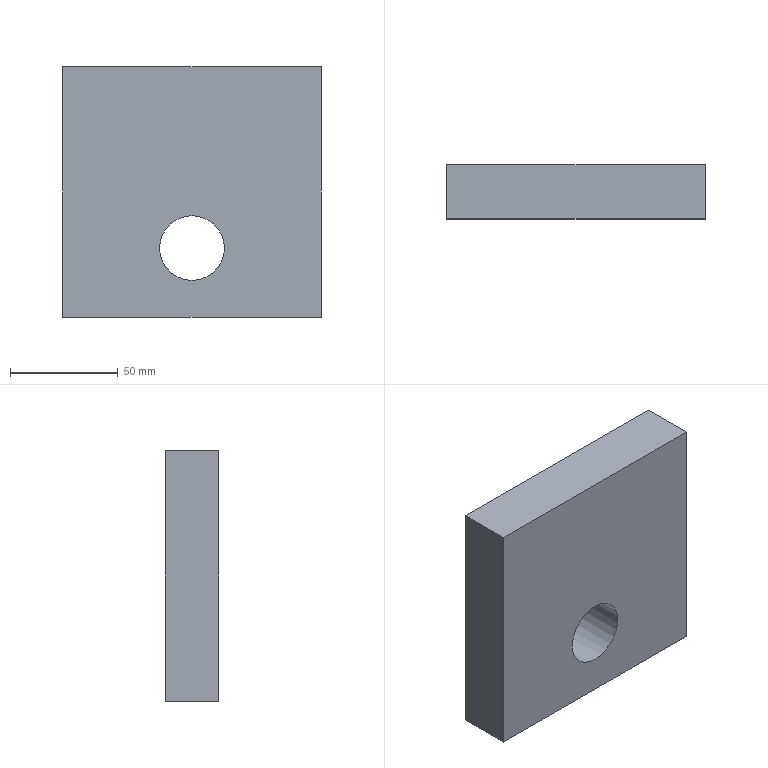Part | NX | features 掩护梁 2 | 1 solid | 7 faces | box 120 x 25 x 116 mm | volume 330329 mm3 | plane 6 | cylinder 1 | commonest cylinder face diameters 30 x1
STEP:
#1=CARTESIAN_POINT('',(-1641.68,3664.947,-172.771));
#2=VERTEX_POINT('',#1);
#3=CARTESIAN_POINT('',(-1641.68,3689.947,-172.771));
#4=VERTEX_POINT('',#3);
#5=CARTESIAN_POINT('',(-1641.68,3689.947,-172.771));
#6=DIRECTION('',(0.,1.,0.));
#7=VECTOR('',#6,1000.);
#8=LINE('',#5,#7);
#9=EDGE_CURVE('',#2,#4,#8,.T.);
#10=ORIENTED_EDGE('',*,*,#9,.F.);
#11=CARTESIAN_POINT('',(-1641.68,3664.947,-288.771));
#12=VERTEX_POINT('',#11);
#13=CARTESIAN_POINT('',(-1641.68,3664.947,-288.771));
#14=DIRECTION('',(0.,0.,1.));
#15=VECTOR('',#14,1000.);
#16=LINE('',#13,#15);
#17=EDGE_CURVE('',#12,#2,#16,.T.);
#18=ORIENTED_EDGE('',*,*,#17,.F.);
#19=CARTESIAN_POINT('',(-1641.68,3689.947,-288.771));
#20=VERTEX_POINT('',#19);
#21=CARTESIAN_POINT('',(-1641.68,3689.947,-288.771));
#22=DIRECTION('',(0.,1.,0.));
#23=VECTOR('',#22,1000.);
#24=LINE('',#21,#23);
#25=EDGE_CURVE('',#12,#20,#24,.T.);
#26=ORIENTED_EDGE('',*,*,#25,.T.);
#27=CARTESIAN_POINT('',(-1641.68,3689.947,-288.771));
#28=DIRECTION('',(0.,0.,1.));
#29=VECTOR('',#28,1000.);
#30=LINE('',#27,#29);
#31=EDGE_CURVE('',#20,#4,#30,.T.);
#32=ORIENTED_EDGE('',*,*,#31,.T.);
#33=EDGE_LOOP('',(#10,#18,#26,#32));
#34=FACE_BOUND('',#33,.T.);
#35=CARTESIAN_POINT('',(-1641.68,3689.947,-288.771));
#36=DIRECTION('',(1.,0.,0.));
#37=DIRECTION('',(0.,0.,-1.));
#38=AXIS2_PLACEMENT_3D('',#35,#36,#37);
#39=PLANE('',#38);
#40=ADVANCED_FACE('',(#34),#39,.T.);
#41=CARTESIAN_POINT('',(-1701.68,3664.947,-271.771));
#42=VERTEX_POINT('',#41);
#43=CARTESIAN_POINT('',(-1701.68,3664.947,-256.771));
#44=DIRECTION('',(0.,-1.,0.));
#45=DIRECTION('',(0.,0.,-1.));
#46=AXIS2_PLACEMENT_3D('',#43,#44,#45);
#47=CIRCLE('',#46,15.);
#48=EDGE_CURVE('',#42,#42,#47,.T.);
#49=ORIENTED_EDGE('',*,*,#48,.F.);
#50=EDGE_LOOP('',(#49));
#51=FACE_BOUND('',#50,.T.);
#52=CARTESIAN_POINT('',(-1761.68,3664.947,-172.771));
#53=VERTEX_POINT('',#52);
#54=CARTESIAN_POINT('',(-1641.68,3664.947,-172.771));
#55=DIRECTION('',(1.,0.,0.));
#56=VECTOR('',#55,1000.);
#57=LINE('',#54,#56);
#58=EDGE_CURVE('',#53,#2,#57,.T.);
#59=ORIENTED_EDGE('',*,*,#58,.F.);
#60=CARTESIAN_POINT('',(-1761.68,3664.947,-288.771));
#61=VERTEX_POINT('',#60);
#62=CARTESIAN_POINT('',(-1761.68,3664.947,-288.771));
#63=DIRECTION('',(0.,0.,1.));
#64=VECTOR('',#63,1000.);
#65=LINE('',#62,#64);
#66=EDGE_CURVE('',#61,#53,#65,.T.);
#67=ORIENTED_EDGE('',*,*,#66,.F.);
#68=CARTESIAN_POINT('',(-1641.68,3664.947,-288.771));
#69=DIRECTION('',(1.,0.,0.));
#70=VECTOR('',#69,1000.);
#71=LINE('',#68,#70);
#72=EDGE_CURVE('',#61,#12,#71,.T.);
#73=ORIENTED_EDGE('',*,*,#72,.T.);
#74=ORIENTED_EDGE('',*,*,#17,.T.);
#75=EDGE_LOOP('',(#59,#67,#73,#74));
#76=FACE_BOUND('',#75,.T.);
#77=CARTESIAN_POINT('',(-1641.68,3664.947,-288.771));
#78=DIRECTION('',(0.,-1.,0.));
#79=DIRECTION('',(0.,0.,-1.));
#80=AXIS2_PLACEMENT_3D('',#77,#78,#79);
#81=PLANE('',#80);
#82=ADVANCED_FACE('',(#51,#76),#81,.T.);
#83=CARTESIAN_POINT('',(-1761.68,3689.947,-172.771));
#84=VERTEX_POINT('',#83);
#85=CARTESIAN_POINT('',(-1761.68,3689.947,-172.771));
#86=DIRECTION('',(0.,-1.,0.));
#87=VECTOR('',#86,1000.);
#88=LINE('',#85,#87);
#89=EDGE_CURVE('',#84,#53,#88,.T.);
#90=ORIENTED_EDGE('',*,*,#89,.F.);
#91=CARTESIAN_POINT('',(-1761.68,3689.947,-288.771));
#92=VERTEX_POINT('',#91);
#93=CARTESIAN_POINT('',(-1761.68,3689.947,-288.771));
#94=DIRECTION('',(0.,0.,1.));
#95=VECTOR('',#94,1000.);
#96=LINE('',#93,#95);
#97=EDGE_CURVE('',#92,#84,#96,.T.);
#98=ORIENTED_EDGE('',*,*,#97,.F.);
#99=CARTESIAN_POINT('',(-1761.68,3689.947,-288.771));
#100=DIRECTION('',(0.,-1.,0.));
#101=VECTOR('',#100,1000.);
#102=LINE('',#99,#101);
#103=EDGE_CURVE('',#92,#61,#102,.T.);
#104=ORIENTED_EDGE('',*,*,#103,.T.);
#105=ORIENTED_EDGE('',*,*,#66,.T.);
#106=EDGE_LOOP('',(#90,#98,#104,#105));
#107=FACE_BOUND('',#106,.T.);
#108=CARTESIAN_POINT('',(-1761.68,3689.947,-288.771));
#109=DIRECTION('',(-1.,0.,0.));
#110=DIRECTION('',(0.,0.,1.));
#111=AXIS2_PLACEMENT_3D('',#108,#109,#110);
#112=PLANE('',#111);
#113=ADVANCED_FACE('',(#107),#112,.T.);
#114=CARTESIAN_POINT('',(-1701.68,3689.947,-241.771));
#115=VERTEX_POINT('',#114);
#116=CARTESIAN_POINT('',(-1701.68,3689.947,-256.771));
#117=DIRECTION('',(0.,1.,0.));
#118=DIRECTION('',(0.,0.,1.));
#119=AXIS2_PLACEMENT_3D('',#116,#117,#118);
#120=CIRCLE('',#119,15.);
#121=EDGE_CURVE('',#115,#115,#120,.T.);
#122=ORIENTED_EDGE('',*,*,#121,.F.);
#123=EDGE_LOOP('',(#122));
#124=FACE_BOUND('',#123,.T.);
#125=CARTESIAN_POINT('',(-1641.68,3689.947,-172.771));
#126=DIRECTION('',(-1.,0.,0.));
#127=VECTOR('',#126,1000.);
#128=LINE('',#125,#127);
#129=EDGE_CURVE('',#4,#84,#128,.T.);
#130=ORIENTED_EDGE('',*,*,#129,.F.);
#131=ORIENTED_EDGE('',*,*,#31,.F.);
#132=CARTESIAN_POINT('',(-1641.68,3689.947,-288.771));
#133=DIRECTION('',(-1.,0.,0.));
#134=VECTOR('',#133,1000.);
#135=LINE('',#132,#134);
#136=EDGE_CURVE('',#20,#92,#135,.T.);
#137=ORIENTED_EDGE('',*,*,#136,.T.);
#138=ORIENTED_EDGE('',*,*,#97,.T.);
#139=EDGE_LOOP('',(#130,#131,#137,#138));
#140=FACE_BOUND('',#139,.T.);
#141=CARTESIAN_POINT('',(-1641.68,3689.947,-288.771));
#142=DIRECTION('',(0.,1.,0.));
#143=DIRECTION('',(0.,0.,1.));
#144=AXIS2_PLACEMENT_3D('',#141,#142,#143);
#145=PLANE('',#144);
#146=ADVANCED_FACE('',(#124,#140),#145,.T.);
#147=ORIENTED_EDGE('',*,*,#25,.F.);
#148=ORIENTED_EDGE('',*,*,#72,.F.);
#149=ORIENTED_EDGE('',*,*,#103,.F.);
#150=ORIENTED_EDGE('',*,*,#136,.F.);
#151=EDGE_LOOP('',(#147,#148,#149,#150));
#152=FACE_BOUND('',#151,.T.);
#153=CARTESIAN_POINT('',(-1641.68,3664.947,-288.771));
#154=DIRECTION('',(0.,0.,-1.));
#155=DIRECTION('',(-1.,0.,0.));
#156=AXIS2_PLACEMENT_3D('',#153,#154,#155);
#157=PLANE('',#156);
#158=ADVANCED_FACE('',(#152),#157,.T.);
#159=ORIENTED_EDGE('',*,*,#9,.T.);
#160=ORIENTED_EDGE('',*,*,#129,.T.);
#161=ORIENTED_EDGE('',*,*,#89,.T.);
#162=ORIENTED_EDGE('',*,*,#58,.T.);
#163=EDGE_LOOP('',(#159,#160,#161,#162));
#164=FACE_BOUND('',#163,.T.);
#165=CARTESIAN_POINT('',(-1641.68,3664.947,-172.771));
#166=DIRECTION('',(0.,0.,-1.));
#167=DIRECTION('',(-1.,0.,0.));
#168=AXIS2_PLACEMENT_3D('',#165,#166,#167);
#169=PLANE('',#168);
#170=ADVANCED_FACE('',(#164),#169,.F.);
#171=ORIENTED_EDGE('',*,*,#48,.T.);
#172=EDGE_LOOP('',(#171));
#173=FACE_BOUND('',#172,.T.);
#174=ORIENTED_EDGE('',*,*,#121,.T.);
#175=EDGE_LOOP('',(#174));
#176=FACE_BOUND('',#175,.T.);
#177=CARTESIAN_POINT('',(-1701.68,3614.947,-256.771));
#178=DIRECTION('',(0.,1.,0.));
#179=DIRECTION('',(0.,0.,1.));
#180=AXIS2_PLACEMENT_3D('',#177,#178,#179);
#181=CYLINDRICAL_SURFACE('',#180,15.);
#182=ADVANCED_FACE('',(#173,#176),#181,.F.);
#183=CLOSED_SHELL('',(#40,#82,#113,#146,#158,#170,#182));
#184=MANIFOLD_SOLID_BREP('',#183);
#185=(LENGTH_UNIT()NAMED_UNIT(*)SI_UNIT(.MILLI.,.METRE.));
#186=UNCERTAINTY_MEASURE_WITH_UNIT(LENGTH_MEASURE(0.00001),#185,'','');
#187=(NAMED_UNIT(*)PLANE_ANGLE_UNIT()SI_UNIT($,.RADIAN.));
#188=(NAMED_UNIT(*)SI_UNIT($,.STERADIAN.)SOLID_ANGLE_UNIT());
#189=(GEOMETRIC_REPRESENTATION_CONTEXT(3)GLOBAL_UNCERTAINTY_ASSIGNED_CONTEXT((#186))GLOBAL_UNIT_ASSIGNED_CONTEXT((#185,#187,#188))REPRESENTATION_CONTEXT('',''));
#190=ADVANCED_BREP_SHAPE_REPRESENTATION('',(#184),#189);